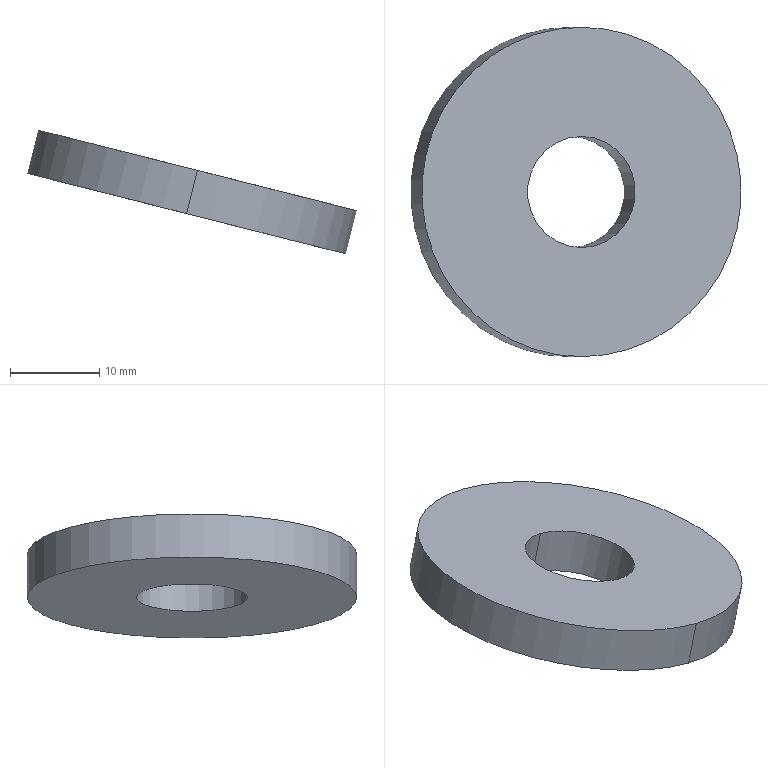Part | SolidWorks | features BaseBody 1 | 1 solid | 6 faces | box 37.096 x 37 x 13.925 mm | volume 4762 mm3 | cylinder 4 | plane 2 | commonest cylinder face diameters 12.5 x2 37 x2
STEP:
#1=CARTESIAN_POINT('',(-479.474,2.25,195.486));
#2=VERTEX_POINT('',#1);
#3=CARTESIAN_POINT('',(-479.474,-10.25,195.486));
#4=VERTEX_POINT('',#3);
#5=CARTESIAN_POINT('',(-479.474,-4.,195.486));
#6=DIRECTION('',(0.2454,0.,0.9694));
#7=DIRECTION('',(-0.9694,0.,0.2454));
#8=AXIS2_PLACEMENT_3D('',#5,#6,#7);
#9=CIRCLE('',#8,6.25);
#10=EDGE_CURVE('',#2,#4,#9,.T.);
#11=ORIENTED_EDGE('',*,*,#10,.T.);
#12=CARTESIAN_POINT('',(-480.701,-10.25,190.638));
#13=VERTEX_POINT('',#12);
#14=CARTESIAN_POINT('',(-479.474,-10.25,195.486));
#15=DIRECTION('',(-0.2454,0.,-0.9694));
#16=VECTOR('',#15,1000.);
#17=LINE('',#14,#16);
#18=EDGE_CURVE('',#4,#13,#17,.T.);
#19=ORIENTED_EDGE('',*,*,#18,.T.);
#20=CARTESIAN_POINT('',(-480.701,2.25,190.638));
#21=VERTEX_POINT('',#20);
#22=CARTESIAN_POINT('',(-480.701,-4.,190.638));
#23=DIRECTION('',(0.2454,0.,0.9694));
#24=DIRECTION('',(-0.9694,0.,0.2454));
#25=AXIS2_PLACEMENT_3D('',#22,#23,#24);
#26=CIRCLE('',#25,6.25);
#27=EDGE_CURVE('',#21,#13,#26,.T.);
#28=ORIENTED_EDGE('',*,*,#27,.F.);
#29=CARTESIAN_POINT('',(-479.474,2.25,195.486));
#30=DIRECTION('',(-0.2454,0.,-0.9694));
#31=VECTOR('',#30,1000.);
#32=LINE('',#29,#31);
#33=EDGE_CURVE('',#2,#21,#32,.T.);
#34=ORIENTED_EDGE('',*,*,#33,.F.);
#35=EDGE_LOOP('',(#11,#19,#28,#34));
#36=FACE_OUTER_BOUND('',#35,.T.);
#37=CARTESIAN_POINT('',(-479.474,-4.,195.486));
#38=DIRECTION('',(-0.2454,0.,-0.9694));
#39=DIRECTION('',(0.,1.,0.));
#40=AXIS2_PLACEMENT_3D('',#37,#38,#39);
#41=CYLINDRICAL_SURFACE('',#40,6.25);
#42=ADVANCED_FACE('',(#36),#41,.F.);
#43=CARTESIAN_POINT('',(-479.474,14.5,195.486));
#44=VERTEX_POINT('',#43);
#45=CARTESIAN_POINT('',(-479.474,-22.5,195.486));
#46=VERTEX_POINT('',#45);
#47=CARTESIAN_POINT('',(-479.474,-4.,195.486));
#48=DIRECTION('',(-0.2454,0.,-0.9694));
#49=DIRECTION('',(0.,1.,0.));
#50=AXIS2_PLACEMENT_3D('',#47,#48,#49);
#51=CIRCLE('',#50,18.5);
#52=EDGE_CURVE('',#44,#46,#51,.T.);
#53=ORIENTED_EDGE('',*,*,#52,.T.);
#54=CARTESIAN_POINT('',(-480.701,-22.5,190.638));
#55=VERTEX_POINT('',#54);
#56=CARTESIAN_POINT('',(-479.474,-22.5,195.486));
#57=DIRECTION('',(-0.2454,0.,-0.9694));
#58=VECTOR('',#57,1000.);
#59=LINE('',#56,#58);
#60=EDGE_CURVE('',#46,#55,#59,.T.);
#61=ORIENTED_EDGE('',*,*,#60,.T.);
#62=CARTESIAN_POINT('',(-480.701,14.5,190.638));
#63=VERTEX_POINT('',#62);
#64=CARTESIAN_POINT('',(-480.701,-4.,190.638));
#65=DIRECTION('',(-0.2454,0.,-0.9694));
#66=DIRECTION('',(0.,1.,0.));
#67=AXIS2_PLACEMENT_3D('',#64,#65,#66);
#68=CIRCLE('',#67,18.5);
#69=EDGE_CURVE('',#63,#55,#68,.T.);
#70=ORIENTED_EDGE('',*,*,#69,.F.);
#71=CARTESIAN_POINT('',(-479.474,14.5,195.486));
#72=DIRECTION('',(-0.2454,0.,-0.9694));
#73=VECTOR('',#72,1000.);
#74=LINE('',#71,#73);
#75=EDGE_CURVE('',#44,#63,#74,.T.);
#76=ORIENTED_EDGE('',*,*,#75,.F.);
#77=EDGE_LOOP('',(#53,#61,#70,#76));
#78=FACE_OUTER_BOUND('',#77,.T.);
#79=CARTESIAN_POINT('',(-479.474,-4.,195.486));
#80=DIRECTION('',(-0.2454,0.,-0.9694));
#81=DIRECTION('',(0.,1.,0.));
#82=AXIS2_PLACEMENT_3D('',#79,#80,#81);
#83=CYLINDRICAL_SURFACE('',#82,18.5);
#84=ADVANCED_FACE('',(#78),#83,.T.);
#85=ORIENTED_EDGE('',*,*,#10,.F.);
#86=CARTESIAN_POINT('',(-479.474,-4.,195.486));
#87=DIRECTION('',(0.2454,0.,0.9694));
#88=DIRECTION('',(-0.9694,0.,0.2454));
#89=AXIS2_PLACEMENT_3D('',#86,#87,#88);
#90=CIRCLE('',#89,6.25);
#91=EDGE_CURVE('',#4,#2,#90,.T.);
#92=ORIENTED_EDGE('',*,*,#91,.F.);
#93=EDGE_LOOP('',(#85,#92));
#94=FACE_BOUND('',#93,.T.);
#95=ORIENTED_EDGE('',*,*,#52,.F.);
#96=CARTESIAN_POINT('',(-479.474,-4.,195.486));
#97=DIRECTION('',(-0.2454,0.,-0.9694));
#98=DIRECTION('',(0.,1.,0.));
#99=AXIS2_PLACEMENT_3D('',#96,#97,#98);
#100=CIRCLE('',#99,18.5);
#101=EDGE_CURVE('',#46,#44,#100,.T.);
#102=ORIENTED_EDGE('',*,*,#101,.F.);
#103=EDGE_LOOP('',(#95,#102));
#104=FACE_OUTER_BOUND('',#103,.T.);
#105=CARTESIAN_POINT('',(-437.132,-66.,184.769));
#106=DIRECTION('',(-0.2454,0.,-0.9694));
#107=DIRECTION('',(-0.9694,0.,0.2454));
#108=AXIS2_PLACEMENT_3D('',#105,#106,#107);
#109=PLANE('',#108);
#110=ADVANCED_FACE('',(#94,#104),#109,.F.);
#111=ORIENTED_EDGE('',*,*,#60,.F.);
#112=ORIENTED_EDGE('',*,*,#101,.T.);
#113=ORIENTED_EDGE('',*,*,#75,.T.);
#114=CARTESIAN_POINT('',(-480.701,-4.,190.638));
#115=DIRECTION('',(-0.2454,0.,-0.9694));
#116=DIRECTION('',(0.,1.,0.));
#117=AXIS2_PLACEMENT_3D('',#114,#115,#116);
#118=CIRCLE('',#117,18.5);
#119=EDGE_CURVE('',#55,#63,#118,.T.);
#120=ORIENTED_EDGE('',*,*,#119,.F.);
#121=EDGE_LOOP('',(#111,#112,#113,#120));
#122=FACE_OUTER_BOUND('',#121,.T.);
#123=CARTESIAN_POINT('',(-479.474,-4.,195.486));
#124=DIRECTION('',(-0.2454,0.,-0.9694));
#125=DIRECTION('',(0.,1.,0.));
#126=AXIS2_PLACEMENT_3D('',#123,#124,#125);
#127=CYLINDRICAL_SURFACE('',#126,18.5);
#128=ADVANCED_FACE('',(#122),#127,.T.);
#129=ORIENTED_EDGE('',*,*,#27,.T.);
#130=CARTESIAN_POINT('',(-480.701,-4.,190.638));
#131=DIRECTION('',(0.2454,0.,0.9694));
#132=DIRECTION('',(-0.9694,0.,0.2454));
#133=AXIS2_PLACEMENT_3D('',#130,#131,#132);
#134=CIRCLE('',#133,6.25);
#135=EDGE_CURVE('',#13,#21,#134,.T.);
#136=ORIENTED_EDGE('',*,*,#135,.T.);
#137=EDGE_LOOP('',(#129,#136));
#138=FACE_BOUND('',#137,.T.);
#139=ORIENTED_EDGE('',*,*,#69,.T.);
#140=ORIENTED_EDGE('',*,*,#119,.T.);
#141=EDGE_LOOP('',(#139,#140));
#142=FACE_OUTER_BOUND('',#141,.T.);
#143=CARTESIAN_POINT('',(-438.359,-66.,179.922));
#144=DIRECTION('',(-0.2454,0.,-0.9694));
#145=DIRECTION('',(-0.9694,0.,0.2454));
#146=AXIS2_PLACEMENT_3D('',#143,#144,#145);
#147=PLANE('',#146);
#148=ADVANCED_FACE('',(#138,#142),#147,.T.);
#149=ORIENTED_EDGE('',*,*,#18,.F.);
#150=ORIENTED_EDGE('',*,*,#91,.T.);
#151=ORIENTED_EDGE('',*,*,#33,.T.);
#152=ORIENTED_EDGE('',*,*,#135,.F.);
#153=EDGE_LOOP('',(#149,#150,#151,#152));
#154=FACE_OUTER_BOUND('',#153,.T.);
#155=CARTESIAN_POINT('',(-479.474,-4.,195.486));
#156=DIRECTION('',(-0.2454,0.,-0.9694));
#157=DIRECTION('',(0.,1.,0.));
#158=AXIS2_PLACEMENT_3D('',#155,#156,#157);
#159=CYLINDRICAL_SURFACE('',#158,6.25);
#160=ADVANCED_FACE('',(#154),#159,.F.);
#161=CLOSED_SHELL('',(#42,#84,#110,#128,#148,#160));
#162=MANIFOLD_SOLID_BREP('',#161);
#163=CARTESIAN_POINT('',(0.,0.,0.));
#164=DIRECTION('',(0.,0.,1.));
#165=DIRECTION('',(1.,0.,0.));
#166=AXIS2_PLACEMENT_3D('',#163,#164,#165);
#167=(LENGTH_UNIT()NAMED_UNIT(*)SI_UNIT(.MILLI.,.METRE.));
#168=UNCERTAINTY_MEASURE_WITH_UNIT(LENGTH_MEASURE(0.00001),#167,'','');
#169=(NAMED_UNIT(*)PLANE_ANGLE_UNIT()SI_UNIT($,.RADIAN.));
#170=(NAMED_UNIT(*)SI_UNIT($,.STERADIAN.)SOLID_ANGLE_UNIT());
#171=(GEOMETRIC_REPRESENTATION_CONTEXT(3)GLOBAL_UNCERTAINTY_ASSIGNED_CONTEXT((#168))GLOBAL_UNIT_ASSIGNED_CONTEXT((#167,#169,#170))REPRESENTATION_CONTEXT('',''));
#172=ADVANCED_BREP_SHAPE_REPRESENTATION('',(#162,#166),#171);